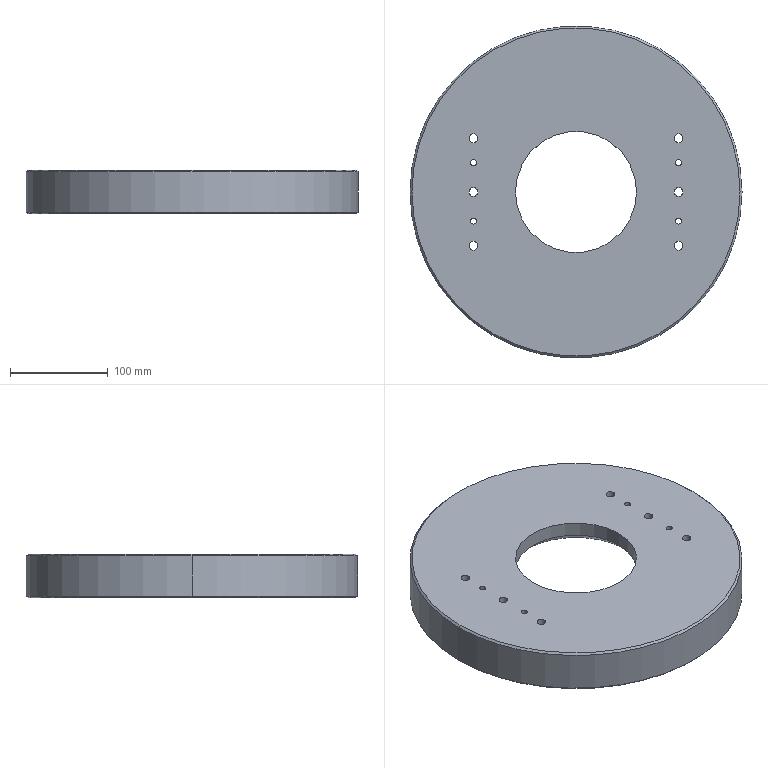NC program | NX | posted with a generic post | part box 340 x 340 x 45 mm
Lines 1 to 147 of 19805:
N10 G17 G21 G94 G90
(FLOOR_WALL , TOOL : D63)
N12 T01 M6
N14 G54
N16 G17 G0 G90 X-115.896 Y175.725 S6500 M3
N18 G43 Z75. H1
N20 Z50.
N22 G94 G1 Z47. F1250.
N24 X-110.348
N26 X110.356
N28 G2 X122.845 Y167.23 R206.552
N30 X147.422 Y146.041 R206.277
N32 G1 X-147.412
N34 G3 X-167.401 Y122.612 R206.653
N36 X-170.222 Y118.659 R206.679
N38 X-171.806 Y116.357 R206.157
N40 G1 X171.809
N42 G2 X174.379 Y112.466 R204.219
N44 X185.632 Y92.728 R206.122
N46 X188.533 Y86.673 R205.361
N48 G1 X-188.533
N50 G3 X-199.528 Y56.99 R206.803
N52 G1 X199.52
N54 G2 X199.67 Y56.46 R208.347
N56 X200.787 Y52.354 R206.082
N58 X204.532 Y34.96 R205.989
N60 G1 X204.55 Y34.858
N62 G2 X205.193 Y30.864 R205.863
N64 X205.698 Y27.306 R206.377
N66 G1 X-205.699
N68 G3 X-205.928 Y25.521 R205.759
N70 X-207.49 Y2.494 R206.347
N72 G1 Y-2.364
N74 Y-2.378
N76 X207.489
N78 G2 X206.941 Y-15.257 R204.872
N80 X205.017 Y-32.061 R206.581
N82 G1 X-205.012
N84 G3 X-198.105 Y-61.745 R207.207
N86 G1 X198.106
N88 G2 X195.356 Y-69.946 R206.581
N90 X186.582 Y-90.797 R205.805
N92 X186.274 Y-91.429 R206.923
N94 G1 X-186.271
N96 G3 X-168.506 Y-121.113 R207.087
N98 G1 X168.492
N100 G2 X166.57 Y-123.74 R205.053
N102 X156.454 Y-136.313 R205.29
N104 X142.557 Y-150.796 R206.323
N106 G1 X-142.538
N108 X-146.872
N110 Z50.
N112 G0 Z75.
N114 X-115.913 Y175.713
N116 Z49.
N118 G1 Z46.
N120 X-110.366
N122 X110.373
N124 G2 X122.749 Y167.3 R206.614
N126 X147.432 Y146.031 R206.277
N128 G1 X-147.422
N130 G3 X-170.222 Y118.659 R206.679
N132 X-171.812 Y116.348 R206.157
N134 G1 X171.816
N136 G2 X174.518 Y112.25 R204.219
N138 X184.16 Y95.619 R206.195
N140 X188.537 Y86.665 R205.361
N142 G1 X-188.537
N144 G3 X-199.529 Y56.983 R206.841
N146 G1 X199.522
N148 G2 X199.67 Y56.46 R208.347
N150 X204.55 Y34.858 R206.082
N152 X205.609 Y27.968 R205.863
N154 X205.699 Y27.3 R206.387
N156 G1 X-205.7
N158 G3 X-206.001 Y24.923 R205.759
N160 X-207.49 Y2.453 R206.415
N162 G1 Y-2.332
N164 X-207.489 Y-2.383
N166 X207.489
N168 G2 X206.901 Y-15.788 R204.872
N170 X205.118 Y-31.37 R205.522
N172 X205.011 Y-32.065 R206.086
N174 G1 X-205.01
N176 G3 X-204.701 Y-33.985 R206.235
N178 X-198.103 Y-61.748 R207.286
N180 G1 X198.107
N182 G2 X186.272 Y-91.431 R206.59
N184 G1 X-186.27
N186 G3 X-168.506 Y-121.113 R207.455
N188 G1 X168.495
N190 G2 X161.219 Y-130.634 R205.763
N192 X142.557 Y-150.796 R206.323
N194 G1 X-142.54
N196 X-146.872
N198 Z49.
N200 G0 Z75.
N202 X-115.913 Y175.713
N204 Z48.
N206 G1 Z45.
N208 X-110.366
N210 X110.373
N212 G2 X122.768 Y167.287 R206.614
N214 X147.431 Y146.031 R206.313
N216 G1 X-147.422
N218 G3 X-170.217 Y118.666 R206.647
N220 X-171.812 Y116.348 R206.106
N222 G1 X171.815
N224 G2 X174.516 Y112.253 R204.288
N226 X184.465 Y95.029 R206.195
N228 X188.537 Y86.665 R205.408
N230 G1 X-188.537
N232 G3 X-199.529 Y56.983 R206.841
N234 G1 X199.522
N236 G2 X199.67 Y56.462 R208.321
N238 X204.55 Y34.858 R206.109
N240 X205.699 Y27.3 R206.38
N242 G1 X-205.7
N244 G3 X-206.002 Y24.916 R205.766
N246 X-207.49 Y2.453 R206.415
N248 G1 Y-2.332
N250 X-207.489 Y-2.383
N252 X207.488
N254 G2 X207.297 Y-9.153 R206.38
N256 X205.01 Y-32.065 R205.393
N258 G1 X-205.01
N260 G3 X-204.718 Y-33.881 R206.266
N262 X-199.869 Y-55.766 R207.286
N264 X-198.105 Y-61.748 R206.602
N266 G1 X198.107
N268 G2 X186.648 Y-90.664 R206.59
N270 X186.274 Y-91.431 R205.195
N272 G1 X-186.273
N274 G3 X-168.491 Y-121.113 R206.04
N276 G1 X168.495
N278 G2 X163.952 Y-127.191 R205.763
N280 X150.566 Y-142.783 R205.363
N282 X142.54 Y-150.796 R207.361
N284 G1 X-142.54
N286 X-146.872
N288 Z48.
N290 G0 Z75.
N292 M5